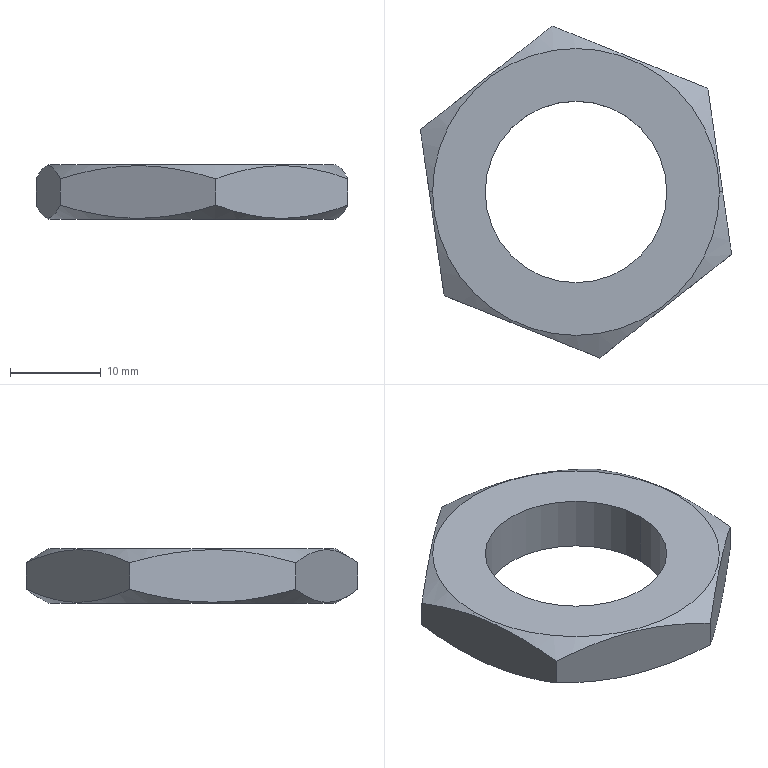Part | SolidWorks | features ICE 2, Extrusion 1 | 1 solid | 14 faces | box 34.301 x 36.575 x 6 mm | volume 3343 mm3 | plane 8 | cone 4 | cylinder 2 | commonest cylinder face diameters 20 x2
STEP:
#1=CARTESIAN_POINT('',(15.8,0.,0.));
#2=VERTEX_POINT('',#1);
#3=CARTESIAN_POINT('',(-15.8,0.,0.));
#4=VERTEX_POINT('',#3);
#5=CARTESIAN_POINT('',(0.,0.,0.));
#6=DIRECTION('',(0.,0.,-1.));
#7=DIRECTION('',(-1.,0.,0.));
#8=AXIS2_PLACEMENT_3D('',#5,#6,#7);
#9=CIRCLE('',#8,15.8);
#10=EDGE_CURVE('',#2,#4,#9,.T.);
#11=ORIENTED_EDGE('',*,*,#10,.F.);
#12=CARTESIAN_POINT('',(16.164,0.,0.2102));
#13=VERTEX_POINT('',#12);
#14=CARTESIAN_POINT('',(15.8,0.,0.));
#15=DIRECTION('',(0.866,0.,0.5));
#16=VECTOR('',#15,1000.);
#17=LINE('',#14,#16);
#18=EDGE_CURVE('',#2,#13,#17,.T.);
#19=ORIENTED_EDGE('',*,*,#18,.T.);
#20=CARTESIAN_POINT('',(17.151,-6.87,1.545));
#21=VERTEX_POINT('',#20);
#22=CARTESIAN_POINT('',(16.164,0.,0.2102));
#23=CARTESIAN_POINT('',(16.499,-2.331,0.4035));
#24=CARTESIAN_POINT('',(16.827,-4.615,0.8869));
#25=CARTESIAN_POINT('',(17.151,-6.87,1.545));
#26=B_SPLINE_CURVE_WITH_KNOTS('',3,(#22,#23,#24,#25),.UNSPECIFIED.,.F.,.F.,(4,4),(0.01162,0.01866),.UNSPECIFIED.);
#27=EDGE_CURVE('',#13,#21,#26,.T.);
#28=ORIENTED_EDGE('',*,*,#27,.T.);
#29=CARTESIAN_POINT('',(2.626,-18.288,1.545));
#30=VERTEX_POINT('',#29);
#31=CARTESIAN_POINT('',(17.151,-6.87,1.545));
#32=CARTESIAN_POINT('',(15.965,-7.802,1.109));
#33=CARTESIAN_POINT('',(14.77,-8.741,0.7503));
#34=CARTESIAN_POINT('',(12.356,-10.638,0.2531));
#35=CARTESIAN_POINT('',(11.137,-11.597,0.1165));
#36=CARTESIAN_POINT('',(9.285,-13.053,0.115));
#37=CARTESIAN_POINT('',(8.664,-13.541,0.1484));
#38=CARTESIAN_POINT('',(7.437,-14.505,0.2786));
#39=CARTESIAN_POINT('',(6.828,-14.984,0.3753));
#40=CARTESIAN_POINT('',(5.01,-16.413,0.7488));
#41=CARTESIAN_POINT('',(3.813,-17.354,1.109));
#42=CARTESIAN_POINT('',(2.626,-18.288,1.545));
#43=B_SPLINE_CURVE_WITH_KNOTS('',3,(#31,#32,#33,#34,#35,#36,#37,#38,#39,#40,#41,#42),.UNSPECIFIED.,.F.,.F.,(4,2,2,2,2,4),(0.000000262,0.004665,0.00933,0.01166,0.01399,0.01866),.UNSPECIFIED.);
#44=EDGE_CURVE('',#21,#30,#43,.T.);
#45=ORIENTED_EDGE('',*,*,#44,.T.);
#46=CARTESIAN_POINT('',(-14.525,-11.418,1.545));
#47=VERTEX_POINT('',#46);
#48=CARTESIAN_POINT('',(2.626,-18.288,1.545));
#49=CARTESIAN_POINT('',(1.226,-17.727,1.109));
#50=CARTESIAN_POINT('',(-0.1846,-17.162,0.7503));
#51=CARTESIAN_POINT('',(-3.035,-16.02,0.2531));
#52=CARTESIAN_POINT('',(-4.475,-15.443,0.1165));
#53=CARTESIAN_POINT('',(-6.662,-14.567,0.115));
#54=CARTESIAN_POINT('',(-7.394,-14.274,0.1484));
#55=CARTESIAN_POINT('',(-8.843,-13.694,0.2786));
#56=CARTESIAN_POINT('',(-9.563,-13.405,0.3753));
#57=CARTESIAN_POINT('',(-11.709,-12.546,0.7488));
#58=CARTESIAN_POINT('',(-13.123,-11.979,1.109));
#59=CARTESIAN_POINT('',(-14.525,-11.418,1.545));
#60=B_SPLINE_CURVE_WITH_KNOTS('',3,(#48,#49,#50,#51,#52,#53,#54,#55,#56,#57,#58,#59),.UNSPECIFIED.,.F.,.F.,(4,2,2,2,2,4),(0.000000222,0.004665,0.00933,0.01166,0.01399,0.01866),.UNSPECIFIED.);
#61=EDGE_CURVE('',#30,#47,#60,.T.);
#62=ORIENTED_EDGE('',*,*,#61,.T.);
#63=CARTESIAN_POINT('',(-16.164,0.,0.2102));
#64=VERTEX_POINT('',#63);
#65=CARTESIAN_POINT('',(-14.525,-11.418,1.545));
#66=CARTESIAN_POINT('',(-14.792,-9.558,1.002));
#67=CARTESIAN_POINT('',(-15.061,-7.681,0.5786));
#68=CARTESIAN_POINT('',(-15.471,-4.827,0.219));
#69=CARTESIAN_POINT('',(-15.609,-3.869,0.1451));
#70=CARTESIAN_POINT('',(-15.886,-1.938,0.1004));
#71=CARTESIAN_POINT('',(-16.026,-0.9626,0.1304));
#72=CARTESIAN_POINT('',(-16.164,0.,0.2102));
#73=B_SPLINE_CURVE_WITH_KNOTS('',3,(#65,#66,#67,#68,#69,#70,#71,#72),.UNSPECIFIED.,.F.,.F.,(4,2,2,4),(0.000000208,0.005811,0.008717,0.01162),.UNSPECIFIED.);
#74=EDGE_CURVE('',#47,#64,#73,.T.);
#75=ORIENTED_EDGE('',*,*,#74,.T.);
#76=CARTESIAN_POINT('',(-15.8,0.,0.));
#77=DIRECTION('',(-0.866,0.,0.5));
#78=VECTOR('',#77,1000.);
#79=LINE('',#76,#78);
#80=EDGE_CURVE('',#4,#64,#79,.T.);
#81=ORIENTED_EDGE('',*,*,#80,.F.);
#82=EDGE_LOOP('',(#11,#19,#28,#45,#62,#75,#81));
#83=FACE_OUTER_BOUND('',#82,.T.);
#84=CARTESIAN_POINT('',(0.,0.,0.));
#85=DIRECTION('',(0.,0.,1.));
#86=DIRECTION('',(-1.,0.,0.));
#87=AXIS2_PLACEMENT_3D('',#84,#85,#86);
#88=CONICAL_SURFACE('',#87,15.8,1.047);
#89=ADVANCED_FACE('',(#83),#88,.T.);
#90=CARTESIAN_POINT('',(-15.8,0.,6.));
#91=VERTEX_POINT('',#90);
#92=CARTESIAN_POINT('',(15.8,0.,6.));
#93=VERTEX_POINT('',#92);
#94=CARTESIAN_POINT('',(0.,0.,6.));
#95=DIRECTION('',(0.,0.,1.));
#96=DIRECTION('',(1.,0.,0.));
#97=AXIS2_PLACEMENT_3D('',#94,#95,#96);
#98=CIRCLE('',#97,15.8);
#99=EDGE_CURVE('',#91,#93,#98,.T.);
#100=ORIENTED_EDGE('',*,*,#99,.F.);
#101=CARTESIAN_POINT('',(-16.164,0.,5.79));
#102=VERTEX_POINT('',#101);
#103=CARTESIAN_POINT('',(-15.8,0.,6.));
#104=DIRECTION('',(-0.866,0.,-0.5));
#105=VECTOR('',#104,1000.);
#106=LINE('',#103,#105);
#107=EDGE_CURVE('',#91,#102,#106,.T.);
#108=ORIENTED_EDGE('',*,*,#107,.T.);
#109=CARTESIAN_POINT('',(-14.525,-11.418,4.455));
#110=VERTEX_POINT('',#109);
#111=CARTESIAN_POINT('',(-16.164,0.,5.79));
#112=CARTESIAN_POINT('',(-16.027,-0.9554,5.869));
#113=CARTESIAN_POINT('',(-15.889,-1.918,5.899));
#114=CARTESIAN_POINT('',(-15.61,-3.857,5.856));
#115=CARTESIAN_POINT('',(-15.472,-4.819,5.782));
#116=CARTESIAN_POINT('',(-15.061,-7.681,5.422));
#117=CARTESIAN_POINT('',(-14.791,-9.559,4.998));
#118=CARTESIAN_POINT('',(-14.525,-11.418,4.455));
#119=B_SPLINE_CURVE_WITH_KNOTS('',3,(#111,#112,#113,#114,#115,#116,#117,#118),.UNSPECIFIED.,.F.,.F.,(4,2,2,4),(0.00706,0.009959,0.01286,0.01866),.UNSPECIFIED.);
#120=EDGE_CURVE('',#102,#110,#119,.T.);
#121=ORIENTED_EDGE('',*,*,#120,.T.);
#122=CARTESIAN_POINT('',(2.626,-18.288,4.455));
#123=VERTEX_POINT('',#122);
#124=CARTESIAN_POINT('',(-14.525,-11.418,4.455));
#125=CARTESIAN_POINT('',(-13.124,-11.979,4.891));
#126=CARTESIAN_POINT('',(-11.714,-12.544,5.25));
#127=CARTESIAN_POINT('',(-8.864,-13.685,5.747));
#128=CARTESIAN_POINT('',(-7.424,-14.262,5.884));
#129=CARTESIAN_POINT('',(-5.237,-15.138,5.885));
#130=CARTESIAN_POINT('',(-4.504,-15.432,5.852));
#131=CARTESIAN_POINT('',(-3.055,-16.012,5.721));
#132=CARTESIAN_POINT('',(-2.336,-16.3,5.625));
#133=CARTESIAN_POINT('',(-0.1896,-17.16,5.251));
#134=CARTESIAN_POINT('',(1.224,-17.726,4.891));
#135=CARTESIAN_POINT('',(2.626,-18.288,4.455));
#136=B_SPLINE_CURVE_WITH_KNOTS('',3,(#124,#125,#126,#127,#128,#129,#130,#131,#132,#133,#134,#135),.UNSPECIFIED.,.F.,.F.,(4,2,2,2,2,4),(0.000000222,0.004665,0.00933,0.01166,0.01399,0.01866),.UNSPECIFIED.);
#137=EDGE_CURVE('',#110,#123,#136,.T.);
#138=ORIENTED_EDGE('',*,*,#137,.T.);
#139=CARTESIAN_POINT('',(17.151,-6.87,4.455));
#140=VERTEX_POINT('',#139);
#141=CARTESIAN_POINT('',(2.626,-18.288,4.455));
#142=CARTESIAN_POINT('',(3.812,-17.355,4.891));
#143=CARTESIAN_POINT('',(5.006,-16.417,5.25));
#144=CARTESIAN_POINT('',(7.42,-14.519,5.747));
#145=CARTESIAN_POINT('',(8.639,-13.56,5.884));
#146=CARTESIAN_POINT('',(10.492,-12.104,5.885));
#147=CARTESIAN_POINT('',(11.112,-11.617,5.852));
#148=CARTESIAN_POINT('',(12.339,-10.652,5.721));
#149=CARTESIAN_POINT('',(12.949,-10.173,5.625));
#150=CARTESIAN_POINT('',(14.766,-8.744,5.251));
#151=CARTESIAN_POINT('',(15.963,-7.803,4.891));
#152=CARTESIAN_POINT('',(17.151,-6.87,4.455));
#153=B_SPLINE_CURVE_WITH_KNOTS('',3,(#141,#142,#143,#144,#145,#146,#147,#148,#149,#150,#151,#152),.UNSPECIFIED.,.F.,.F.,(4,2,2,2,2,4),(0.000000262,0.004665,0.00933,0.01166,0.01399,0.01866),.UNSPECIFIED.);
#154=EDGE_CURVE('',#123,#140,#153,.T.);
#155=ORIENTED_EDGE('',*,*,#154,.T.);
#156=CARTESIAN_POINT('',(16.164,0.,5.79));
#157=VERTEX_POINT('',#156);
#158=CARTESIAN_POINT('',(17.151,-6.87,4.455));
#159=CARTESIAN_POINT('',(16.826,-4.61,5.114));
#160=CARTESIAN_POINT('',(16.498,-2.326,5.597));
#161=CARTESIAN_POINT('',(16.164,0.,5.79));
#162=B_SPLINE_CURVE_WITH_KNOTS('',3,(#158,#159,#160,#161),.UNSPECIFIED.,.F.,.F.,(4,4),(0.000000208,0.00706),.UNSPECIFIED.);
#163=EDGE_CURVE('',#140,#157,#162,.T.);
#164=ORIENTED_EDGE('',*,*,#163,.T.);
#165=CARTESIAN_POINT('',(15.8,0.,6.));
#166=DIRECTION('',(0.866,0.,-0.5));
#167=VECTOR('',#166,1000.);
#168=LINE('',#165,#167);
#169=EDGE_CURVE('',#93,#157,#168,.T.);
#170=ORIENTED_EDGE('',*,*,#169,.F.);
#171=EDGE_LOOP('',(#100,#108,#121,#138,#155,#164,#170));
#172=FACE_OUTER_BOUND('',#171,.T.);
#173=CARTESIAN_POINT('',(0.,0.,6.));
#174=DIRECTION('',(0.,0.,-1.));
#175=DIRECTION('',(1.,0.,0.));
#176=AXIS2_PLACEMENT_3D('',#173,#174,#175);
#177=CONICAL_SURFACE('',#176,15.8,1.047);
#178=ADVANCED_FACE('',(#172),#177,.T.);
#179=CARTESIAN_POINT('',(-10.,0.,6.));
#180=VERTEX_POINT('',#179);
#181=CARTESIAN_POINT('',(10.,0.,6.));
#182=VERTEX_POINT('',#181);
#183=CARTESIAN_POINT('',(0.,0.,6.));
#184=DIRECTION('',(0.,0.,1.));
#185=DIRECTION('',(1.,0.,0.));
#186=AXIS2_PLACEMENT_3D('',#183,#184,#185);
#187=CIRCLE('',#186,10.);
#188=EDGE_CURVE('',#180,#182,#187,.T.);
#189=ORIENTED_EDGE('',*,*,#188,.T.);
#190=CARTESIAN_POINT('',(10.,0.,0.));
#191=VERTEX_POINT('',#190);
#192=CARTESIAN_POINT('',(10.,0.,6.));
#193=DIRECTION('',(0.,0.,-1.));
#194=VECTOR('',#193,1000.);
#195=LINE('',#192,#194);
#196=EDGE_CURVE('',#182,#191,#195,.T.);
#197=ORIENTED_EDGE('',*,*,#196,.T.);
#198=CARTESIAN_POINT('',(-10.,0.,0.));
#199=VERTEX_POINT('',#198);
#200=CARTESIAN_POINT('',(0.,0.,0.));
#201=DIRECTION('',(0.,0.,1.));
#202=DIRECTION('',(1.,0.,0.));
#203=AXIS2_PLACEMENT_3D('',#200,#201,#202);
#204=CIRCLE('',#203,10.);
#205=EDGE_CURVE('',#199,#191,#204,.T.);
#206=ORIENTED_EDGE('',*,*,#205,.F.);
#207=CARTESIAN_POINT('',(-10.,0.,6.));
#208=DIRECTION('',(0.,0.,-1.));
#209=VECTOR('',#208,1000.);
#210=LINE('',#207,#209);
#211=EDGE_CURVE('',#180,#199,#210,.T.);
#212=ORIENTED_EDGE('',*,*,#211,.F.);
#213=EDGE_LOOP('',(#189,#197,#206,#212));
#214=FACE_OUTER_BOUND('',#213,.T.);
#215=CARTESIAN_POINT('',(0.,0.,6.));
#216=DIRECTION('',(0.,0.,-1.));
#217=DIRECTION('',(-1.,0.,0.));
#218=AXIS2_PLACEMENT_3D('',#215,#216,#217);
#219=CYLINDRICAL_SURFACE('',#218,10.);
#220=ADVANCED_FACE('',(#214),#219,.F.);
#221=ORIENTED_EDGE('',*,*,#74,.F.);
#222=CARTESIAN_POINT('',(-14.525,-11.418,6.));
#223=DIRECTION('',(0.,0.,-1.));
#224=VECTOR('',#223,1000.);
#225=LINE('',#222,#224);
#226=EDGE_CURVE('',#110,#47,#225,.T.);
#227=ORIENTED_EDGE('',*,*,#226,.F.);
#228=ORIENTED_EDGE('',*,*,#120,.F.);
#229=CARTESIAN_POINT('',(-17.151,6.87,4.455));
#230=VERTEX_POINT('',#229);
#231=CARTESIAN_POINT('',(-17.151,6.87,4.455));
#232=CARTESIAN_POINT('',(-16.826,4.61,5.114));
#233=CARTESIAN_POINT('',(-16.498,2.326,5.597));
#234=CARTESIAN_POINT('',(-16.164,0.,5.79));
#235=B_SPLINE_CURVE_WITH_KNOTS('',3,(#231,#232,#233,#234),.UNSPECIFIED.,.F.,.F.,(4,4),(0.000000208,0.00706),.UNSPECIFIED.);
#236=EDGE_CURVE('',#230,#102,#235,.T.);
#237=ORIENTED_EDGE('',*,*,#236,.F.);
#238=CARTESIAN_POINT('',(-17.151,6.87,1.545));
#239=VERTEX_POINT('',#238);
#240=CARTESIAN_POINT('',(-17.151,6.87,6.));
#241=DIRECTION('',(0.,0.,-1.));
#242=VECTOR('',#241,1000.);
#243=LINE('',#240,#242);
#244=EDGE_CURVE('',#230,#239,#243,.T.);
#245=ORIENTED_EDGE('',*,*,#244,.T.);
#246=CARTESIAN_POINT('',(-16.164,0.,0.2102));
#247=CARTESIAN_POINT('',(-16.499,2.331,0.4035));
#248=CARTESIAN_POINT('',(-16.827,4.615,0.8869));
#249=CARTESIAN_POINT('',(-17.151,6.87,1.545));
#250=B_SPLINE_CURVE_WITH_KNOTS('',3,(#246,#247,#248,#249),.UNSPECIFIED.,.F.,.F.,(4,4),(0.01162,0.01866),.UNSPECIFIED.);
#251=EDGE_CURVE('',#64,#239,#250,.T.);
#252=ORIENTED_EDGE('',*,*,#251,.F.);
#253=EDGE_LOOP('',(#221,#227,#228,#237,#245,#252));
#254=FACE_OUTER_BOUND('',#253,.T.);
#255=CARTESIAN_POINT('',(-17.151,6.87,6.));
#256=DIRECTION('',(0.9898,0.1421,0.));
#257=DIRECTION('',(-0.1421,0.9898,0.));
#258=AXIS2_PLACEMENT_3D('',#255,#256,#257);
#259=PLANE('',#258);
#260=ADVANCED_FACE('',(#254),#259,.F.);
#261=ORIENTED_EDGE('',*,*,#61,.F.);
#262=CARTESIAN_POINT('',(2.626,-18.288,6.));
#263=DIRECTION('',(0.,0.,-1.));
#264=VECTOR('',#263,1000.);
#265=LINE('',#262,#264);
#266=EDGE_CURVE('',#123,#30,#265,.T.);
#267=ORIENTED_EDGE('',*,*,#266,.F.);
#268=ORIENTED_EDGE('',*,*,#137,.F.);
#269=ORIENTED_EDGE('',*,*,#226,.T.);
#270=EDGE_LOOP('',(#261,#267,#268,#269));
#271=FACE_OUTER_BOUND('',#270,.T.);
#272=CARTESIAN_POINT('',(-14.525,-11.418,6.));
#273=DIRECTION('',(0.3718,0.9283,0.));
#274=DIRECTION('',(-0.9283,0.3718,0.));
#275=AXIS2_PLACEMENT_3D('',#272,#273,#274);
#276=PLANE('',#275);
#277=ADVANCED_FACE('',(#271),#276,.F.);
#278=ORIENTED_EDGE('',*,*,#44,.F.);
#279=CARTESIAN_POINT('',(17.151,-6.87,6.));
#280=DIRECTION('',(0.,0.,-1.));
#281=VECTOR('',#280,1000.);
#282=LINE('',#279,#281);
#283=EDGE_CURVE('',#140,#21,#282,.T.);
#284=ORIENTED_EDGE('',*,*,#283,.F.);
#285=ORIENTED_EDGE('',*,*,#154,.F.);
#286=ORIENTED_EDGE('',*,*,#266,.T.);
#287=EDGE_LOOP('',(#278,#284,#285,#286));
#288=FACE_OUTER_BOUND('',#287,.T.);
#289=CARTESIAN_POINT('',(2.626,-18.288,6.));
#290=DIRECTION('',(-0.618,0.7862,0.));
#291=DIRECTION('',(-0.7862,-0.618,0.));
#292=AXIS2_PLACEMENT_3D('',#289,#290,#291);
#293=PLANE('',#292);
#294=ADVANCED_FACE('',(#288),#293,.F.);
#295=CARTESIAN_POINT('',(14.525,11.418,1.545));
#296=VERTEX_POINT('',#295);
#297=CARTESIAN_POINT('',(14.525,11.418,1.545));
#298=CARTESIAN_POINT('',(14.792,9.558,1.002));
#299=CARTESIAN_POINT('',(15.061,7.681,0.5786));
#300=CARTESIAN_POINT('',(15.471,4.827,0.219));
#301=CARTESIAN_POINT('',(15.609,3.869,0.1451));
#302=CARTESIAN_POINT('',(15.886,1.938,0.1004));
#303=CARTESIAN_POINT('',(16.026,0.9626,0.1304));
#304=CARTESIAN_POINT('',(16.164,0.,0.2102));
#305=B_SPLINE_CURVE_WITH_KNOTS('',3,(#297,#298,#299,#300,#301,#302,#303,#304),.UNSPECIFIED.,.F.,.F.,(4,2,2,4),(0.000000208,0.005811,0.008717,0.01162),.UNSPECIFIED.);
#306=EDGE_CURVE('',#296,#13,#305,.T.);
#307=ORIENTED_EDGE('',*,*,#306,.F.);
#308=CARTESIAN_POINT('',(14.525,11.418,4.455));
#309=VERTEX_POINT('',#308);
#310=CARTESIAN_POINT('',(14.525,11.418,6.));
#311=DIRECTION('',(0.,0.,-1.));
#312=VECTOR('',#311,1000.);
#313=LINE('',#310,#312);
#314=EDGE_CURVE('',#309,#296,#313,.T.);
#315=ORIENTED_EDGE('',*,*,#314,.F.);
#316=CARTESIAN_POINT('',(16.164,0.,5.79));
#317=CARTESIAN_POINT('',(16.027,0.9554,5.869));
#318=CARTESIAN_POINT('',(15.889,1.918,5.899));
#319=CARTESIAN_POINT('',(15.61,3.857,5.856));
#320=CARTESIAN_POINT('',(15.472,4.819,5.782));
#321=CARTESIAN_POINT('',(15.061,7.681,5.422));
#322=CARTESIAN_POINT('',(14.791,9.559,4.998));
#323=CARTESIAN_POINT('',(14.525,11.418,4.455));
#324=B_SPLINE_CURVE_WITH_KNOTS('',3,(#316,#317,#318,#319,#320,#321,#322,#323),.UNSPECIFIED.,.F.,.F.,(4,2,2,4),(0.00706,0.009959,0.01286,0.01866),.UNSPECIFIED.);
#325=EDGE_CURVE('',#157,#309,#324,.T.);
#326=ORIENTED_EDGE('',*,*,#325,.F.);
#327=ORIENTED_EDGE('',*,*,#163,.F.);
#328=ORIENTED_EDGE('',*,*,#283,.T.);
#329=ORIENTED_EDGE('',*,*,#27,.F.);
#330=EDGE_LOOP('',(#307,#315,#326,#327,#328,#329));
#331=FACE_OUTER_BOUND('',#330,.T.);
#332=CARTESIAN_POINT('',(17.151,-6.87,6.));
#333=DIRECTION('',(-0.9898,-0.1421,0.));
#334=DIRECTION('',(0.1421,-0.9898,0.));
#335=AXIS2_PLACEMENT_3D('',#332,#333,#334);
#336=PLANE('',#335);
#337=ADVANCED_FACE('',(#331),#336,.F.);
#338=CARTESIAN_POINT('',(-2.626,18.288,1.545));
#339=VERTEX_POINT('',#338);
#340=CARTESIAN_POINT('',(-2.626,18.288,1.545));
#341=CARTESIAN_POINT('',(-1.226,17.727,1.109));
#342=CARTESIAN_POINT('',(0.1846,17.162,0.7503));
#343=CARTESIAN_POINT('',(3.035,16.02,0.2531));
#344=CARTESIAN_POINT('',(4.475,15.443,0.1165));
#345=CARTESIAN_POINT('',(6.662,14.567,0.115));
#346=CARTESIAN_POINT('',(7.394,14.274,0.1484));
#347=CARTESIAN_POINT('',(8.843,13.694,0.2786));
#348=CARTESIAN_POINT('',(9.563,13.405,0.3753));
#349=CARTESIAN_POINT('',(11.709,12.546,0.7488));
#350=CARTESIAN_POINT('',(13.123,11.979,1.109));
#351=CARTESIAN_POINT('',(14.525,11.418,1.545));
#352=B_SPLINE_CURVE_WITH_KNOTS('',3,(#340,#341,#342,#343,#344,#345,#346,#347,#348,#349,#350,#351),.UNSPECIFIED.,.F.,.F.,(4,2,2,2,2,4),(0.000000222,0.004665,0.00933,0.01166,0.01399,0.01866),.UNSPECIFIED.);
#353=EDGE_CURVE('',#339,#296,#352,.T.);
#354=ORIENTED_EDGE('',*,*,#353,.F.);
#355=CARTESIAN_POINT('',(-2.626,18.288,4.455));
#356=VERTEX_POINT('',#355);
#357=CARTESIAN_POINT('',(-2.626,18.288,6.));
#358=DIRECTION('',(0.,0.,-1.));
#359=VECTOR('',#358,1000.);
#360=LINE('',#357,#359);
#361=EDGE_CURVE('',#356,#339,#360,.T.);
#362=ORIENTED_EDGE('',*,*,#361,.F.);
#363=CARTESIAN_POINT('',(14.525,11.418,4.455));
#364=CARTESIAN_POINT('',(13.124,11.979,4.891));
#365=CARTESIAN_POINT('',(11.714,12.544,5.25));
#366=CARTESIAN_POINT('',(8.864,13.685,5.747));
#367=CARTESIAN_POINT('',(7.424,14.262,5.884));
#368=CARTESIAN_POINT('',(5.237,15.138,5.885));
#369=CARTESIAN_POINT('',(4.504,15.432,5.852));
#370=CARTESIAN_POINT('',(3.055,16.012,5.721));
#371=CARTESIAN_POINT('',(2.336,16.3,5.625));
#372=CARTESIAN_POINT('',(0.1896,17.16,5.251));
#373=CARTESIAN_POINT('',(-1.224,17.726,4.891));
#374=CARTESIAN_POINT('',(-2.626,18.288,4.455));
#375=B_SPLINE_CURVE_WITH_KNOTS('',3,(#363,#364,#365,#366,#367,#368,#369,#370,#371,#372,#373,#374),.UNSPECIFIED.,.F.,.F.,(4,2,2,2,2,4),(0.000000222,0.004665,0.00933,0.01166,0.01399,0.01866),.UNSPECIFIED.);
#376=EDGE_CURVE('',#309,#356,#375,.T.);
#377=ORIENTED_EDGE('',*,*,#376,.F.);
#378=ORIENTED_EDGE('',*,*,#314,.T.);
#379=EDGE_LOOP('',(#354,#362,#377,#378));
#380=FACE_OUTER_BOUND('',#379,.T.);
#381=CARTESIAN_POINT('',(14.525,11.418,6.));
#382=DIRECTION('',(-0.3718,-0.9283,0.));
#383=DIRECTION('',(0.9283,-0.3718,0.));
#384=AXIS2_PLACEMENT_3D('',#381,#382,#383);
#385=PLANE('',#384);
#386=ADVANCED_FACE('',(#380),#385,.F.);
#387=CARTESIAN_POINT('',(-17.151,6.87,1.545));
#388=CARTESIAN_POINT('',(-15.965,7.802,1.109));
#389=CARTESIAN_POINT('',(-14.77,8.741,0.7503));
#390=CARTESIAN_POINT('',(-12.356,10.638,0.2531));
#391=CARTESIAN_POINT('',(-11.137,11.597,0.1165));
#392=CARTESIAN_POINT('',(-9.285,13.053,0.115));
#393=CARTESIAN_POINT('',(-8.664,13.541,0.1484));
#394=CARTESIAN_POINT('',(-7.437,14.505,0.2786));
#395=CARTESIAN_POINT('',(-6.828,14.984,0.3753));
#396=CARTESIAN_POINT('',(-5.01,16.413,0.7488));
#397=CARTESIAN_POINT('',(-3.813,17.354,1.109));
#398=CARTESIAN_POINT('',(-2.626,18.288,1.545));
#399=B_SPLINE_CURVE_WITH_KNOTS('',3,(#387,#388,#389,#390,#391,#392,#393,#394,#395,#396,#397,#398),.UNSPECIFIED.,.F.,.F.,(4,2,2,2,2,4),(0.000000262,0.004665,0.00933,0.01166,0.01399,0.01866),.UNSPECIFIED.);
#400=EDGE_CURVE('',#239,#339,#399,.T.);
#401=ORIENTED_EDGE('',*,*,#400,.F.);
#402=ORIENTED_EDGE('',*,*,#244,.F.);
#403=CARTESIAN_POINT('',(-2.626,18.288,4.455));
#404=CARTESIAN_POINT('',(-3.812,17.355,4.891));
#405=CARTESIAN_POINT('',(-5.006,16.417,5.25));
#406=CARTESIAN_POINT('',(-7.42,14.519,5.747));
#407=CARTESIAN_POINT('',(-8.639,13.56,5.884));
#408=CARTESIAN_POINT('',(-10.492,12.104,5.885));
#409=CARTESIAN_POINT('',(-11.112,11.617,5.852));
#410=CARTESIAN_POINT('',(-12.339,10.652,5.721));
#411=CARTESIAN_POINT('',(-12.949,10.173,5.625));
#412=CARTESIAN_POINT('',(-14.766,8.744,5.251));
#413=CARTESIAN_POINT('',(-15.963,7.803,4.891));
#414=CARTESIAN_POINT('',(-17.151,6.87,4.455));
#415=B_SPLINE_CURVE_WITH_KNOTS('',3,(#403,#404,#405,#406,#407,#408,#409,#410,#411,#412,#413,#414),.UNSPECIFIED.,.F.,.F.,(4,2,2,2,2,4),(0.000000262,0.004665,0.00933,0.01166,0.01399,0.01866),.UNSPECIFIED.);
#416=EDGE_CURVE('',#356,#230,#415,.T.);
#417=ORIENTED_EDGE('',*,*,#416,.F.);
#418=ORIENTED_EDGE('',*,*,#361,.T.);
#419=EDGE_LOOP('',(#401,#402,#417,#418));
#420=FACE_OUTER_BOUND('',#419,.T.);
#421=CARTESIAN_POINT('',(-2.626,18.288,6.));
#422=DIRECTION('',(0.618,-0.7862,0.));
#423=DIRECTION('',(0.7862,0.618,0.));
#424=AXIS2_PLACEMENT_3D('',#421,#422,#423);
#425=PLANE('',#424);
#426=ADVANCED_FACE('',(#420),#425,.F.);
#427=ORIENTED_EDGE('',*,*,#205,.T.);
#428=CARTESIAN_POINT('',(0.,0.,0.));
#429=DIRECTION('',(0.,0.,1.));
#430=DIRECTION('',(1.,0.,0.));
#431=AXIS2_PLACEMENT_3D('',#428,#429,#430);
#432=CIRCLE('',#431,10.);
#433=EDGE_CURVE('',#191,#199,#432,.T.);
#434=ORIENTED_EDGE('',*,*,#433,.T.);
#435=EDGE_LOOP('',(#427,#434));
#436=FACE_BOUND('',#435,.T.);
#437=CARTESIAN_POINT('',(0.,0.,0.));
#438=DIRECTION('',(0.,0.,-1.));
#439=DIRECTION('',(-1.,0.,0.));
#440=AXIS2_PLACEMENT_3D('',#437,#438,#439);
#441=CIRCLE('',#440,15.8);
#442=EDGE_CURVE('',#4,#2,#441,.T.);
#443=ORIENTED_EDGE('',*,*,#442,.T.);
#444=ORIENTED_EDGE('',*,*,#10,.T.);
#445=EDGE_LOOP('',(#443,#444));
#446=FACE_OUTER_BOUND('',#445,.T.);
#447=CARTESIAN_POINT('',(0.,0.,0.));
#448=DIRECTION('',(0.,0.,1.));
#449=DIRECTION('',(1.,0.,0.));
#450=AXIS2_PLACEMENT_3D('',#447,#448,#449);
#451=PLANE('',#450);
#452=ADVANCED_FACE('',(#436,#446),#451,.F.);
#453=ORIENTED_EDGE('',*,*,#188,.F.);
#454=CARTESIAN_POINT('',(0.,0.,6.));
#455=DIRECTION('',(0.,0.,1.));
#456=DIRECTION('',(1.,0.,0.));
#457=AXIS2_PLACEMENT_3D('',#454,#455,#456);
#458=CIRCLE('',#457,10.);
#459=EDGE_CURVE('',#182,#180,#458,.T.);
#460=ORIENTED_EDGE('',*,*,#459,.F.);
#461=EDGE_LOOP('',(#453,#460));
#462=FACE_BOUND('',#461,.T.);
#463=CARTESIAN_POINT('',(0.,0.,6.));
#464=DIRECTION('',(0.,0.,1.));
#465=DIRECTION('',(1.,0.,0.));
#466=AXIS2_PLACEMENT_3D('',#463,#464,#465);
#467=CIRCLE('',#466,15.8);
#468=EDGE_CURVE('',#93,#91,#467,.T.);
#469=ORIENTED_EDGE('',*,*,#468,.T.);
#470=ORIENTED_EDGE('',*,*,#99,.T.);
#471=EDGE_LOOP('',(#469,#470));
#472=FACE_OUTER_BOUND('',#471,.T.);
#473=CARTESIAN_POINT('',(0.,0.,6.));
#474=DIRECTION('',(0.,0.,1.));
#475=DIRECTION('',(1.,0.,0.));
#476=AXIS2_PLACEMENT_3D('',#473,#474,#475);
#477=PLANE('',#476);
#478=ADVANCED_FACE('',(#462,#472),#477,.T.);
#479=ORIENTED_EDGE('',*,*,#196,.F.);
#480=ORIENTED_EDGE('',*,*,#459,.T.);
#481=ORIENTED_EDGE('',*,*,#211,.T.);
#482=ORIENTED_EDGE('',*,*,#433,.F.);
#483=EDGE_LOOP('',(#479,#480,#481,#482));
#484=FACE_OUTER_BOUND('',#483,.T.);
#485=CARTESIAN_POINT('',(0.,0.,6.));
#486=DIRECTION('',(0.,0.,-1.));
#487=DIRECTION('',(-1.,0.,0.));
#488=AXIS2_PLACEMENT_3D('',#485,#486,#487);
#489=CYLINDRICAL_SURFACE('',#488,10.);
#490=ADVANCED_FACE('',(#484),#489,.F.);
#491=ORIENTED_EDGE('',*,*,#107,.F.);
#492=ORIENTED_EDGE('',*,*,#468,.F.);
#493=ORIENTED_EDGE('',*,*,#169,.T.);
#494=ORIENTED_EDGE('',*,*,#325,.T.);
#495=ORIENTED_EDGE('',*,*,#376,.T.);
#496=ORIENTED_EDGE('',*,*,#416,.T.);
#497=ORIENTED_EDGE('',*,*,#236,.T.);
#498=EDGE_LOOP('',(#491,#492,#493,#494,#495,#496,#497));
#499=FACE_OUTER_BOUND('',#498,.T.);
#500=CARTESIAN_POINT('',(0.,0.,6.));
#501=DIRECTION('',(0.,0.,-1.));
#502=DIRECTION('',(1.,0.,0.));
#503=AXIS2_PLACEMENT_3D('',#500,#501,#502);
#504=CONICAL_SURFACE('',#503,15.8,1.047);
#505=ADVANCED_FACE('',(#499),#504,.T.);
#506=ORIENTED_EDGE('',*,*,#18,.F.);
#507=ORIENTED_EDGE('',*,*,#442,.F.);
#508=ORIENTED_EDGE('',*,*,#80,.T.);
#509=ORIENTED_EDGE('',*,*,#251,.T.);
#510=ORIENTED_EDGE('',*,*,#400,.T.);
#511=ORIENTED_EDGE('',*,*,#353,.T.);
#512=ORIENTED_EDGE('',*,*,#306,.T.);
#513=EDGE_LOOP('',(#506,#507,#508,#509,#510,#511,#512));
#514=FACE_OUTER_BOUND('',#513,.T.);
#515=CARTESIAN_POINT('',(0.,0.,0.));
#516=DIRECTION('',(0.,0.,1.));
#517=DIRECTION('',(-1.,0.,0.));
#518=AXIS2_PLACEMENT_3D('',#515,#516,#517);
#519=CONICAL_SURFACE('',#518,15.8,1.047);
#520=ADVANCED_FACE('',(#514),#519,.T.);
#521=CLOSED_SHELL('',(#89,#178,#220,#260,#277,#294,#337,#386,#426,#452,#478,#490,#505,#520));
#522=MANIFOLD_SOLID_BREP('',#521);
#523=CARTESIAN_POINT('',(0.,0.,0.));
#524=DIRECTION('',(0.,0.,1.));
#525=DIRECTION('',(1.,0.,0.));
#526=AXIS2_PLACEMENT_3D('',#523,#524,#525);
#527=(LENGTH_UNIT()NAMED_UNIT(*)SI_UNIT(.MILLI.,.METRE.));
#528=UNCERTAINTY_MEASURE_WITH_UNIT(LENGTH_MEASURE(0.00001),#527,'','');
#529=(NAMED_UNIT(*)PLANE_ANGLE_UNIT()SI_UNIT($,.RADIAN.));
#530=(NAMED_UNIT(*)SI_UNIT($,.STERADIAN.)SOLID_ANGLE_UNIT());
#531=(GEOMETRIC_REPRESENTATION_CONTEXT(3)GLOBAL_UNCERTAINTY_ASSIGNED_CONTEXT((#528))GLOBAL_UNIT_ASSIGNED_CONTEXT((#527,#529,#530))REPRESENTATION_CONTEXT('',''));
#532=ADVANCED_BREP_SHAPE_REPRESENTATION('',(#522,#526),#531);